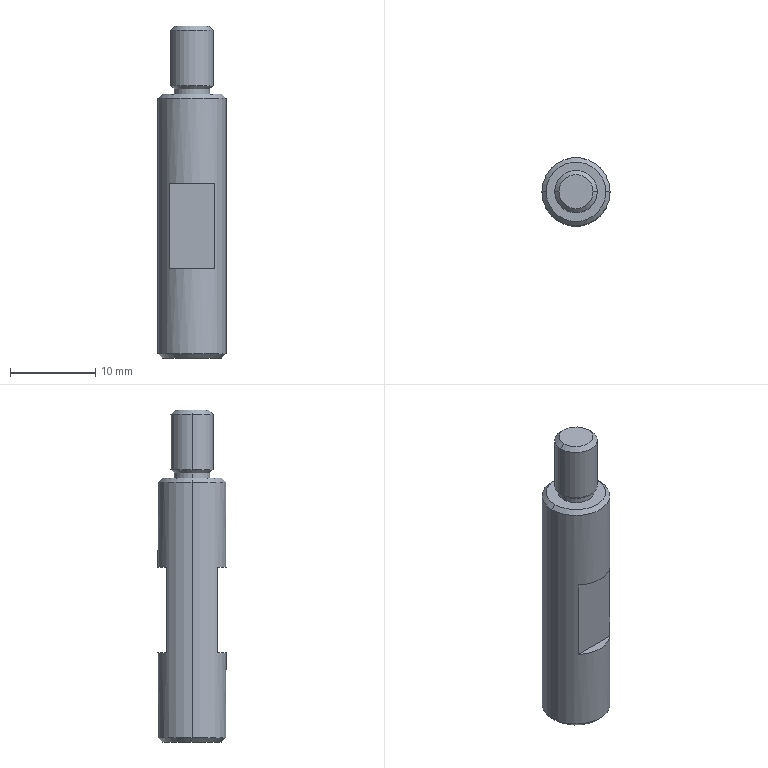Part | STEP file | PN_0014 | 1 solid | 27 faces | box 8 x 8 x 39 mm | volume 1541 mm3 | cone 10 | plane 9 | cylinder 8 | commonest cylinder face diameters 3.3 x2 4.2 x2 5 x2 8 x2